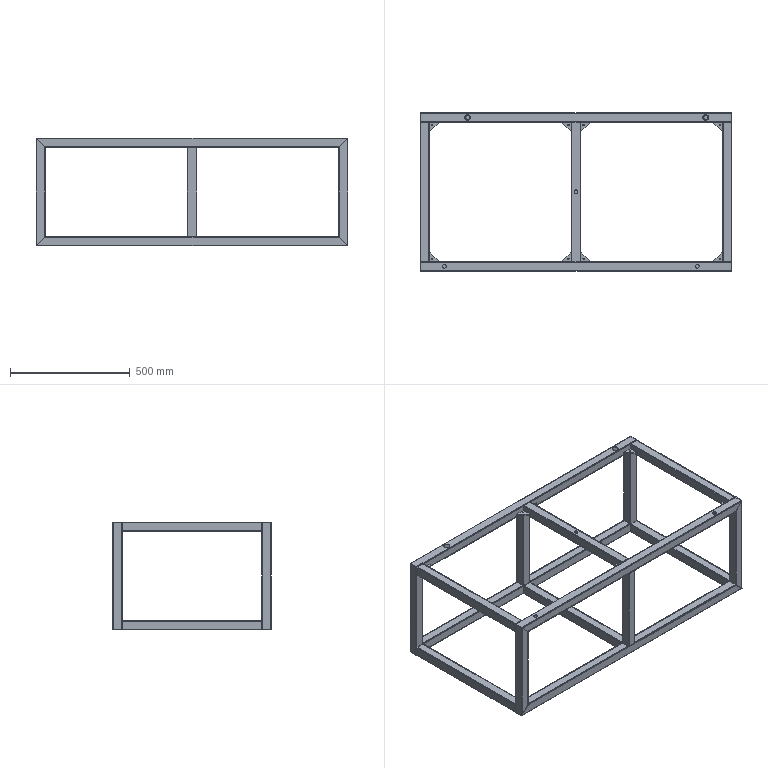Part | SolidWorks | features WeldCornerFeat 9, Gusset 8, ICE 3, WeldMemberFeat 3, 3DProfileFeature 1, HoleWzd 1, WeldmentFeature 1 | 24 solids | 372 faces | box 1300 x 660 x 450 mm | volume 3264516 mm3 | plane 200 | cylinder 172 | commonest cylinder face diameters 2 x64 6 x64 5 x16 16 x16 6.5 x8 25 x4